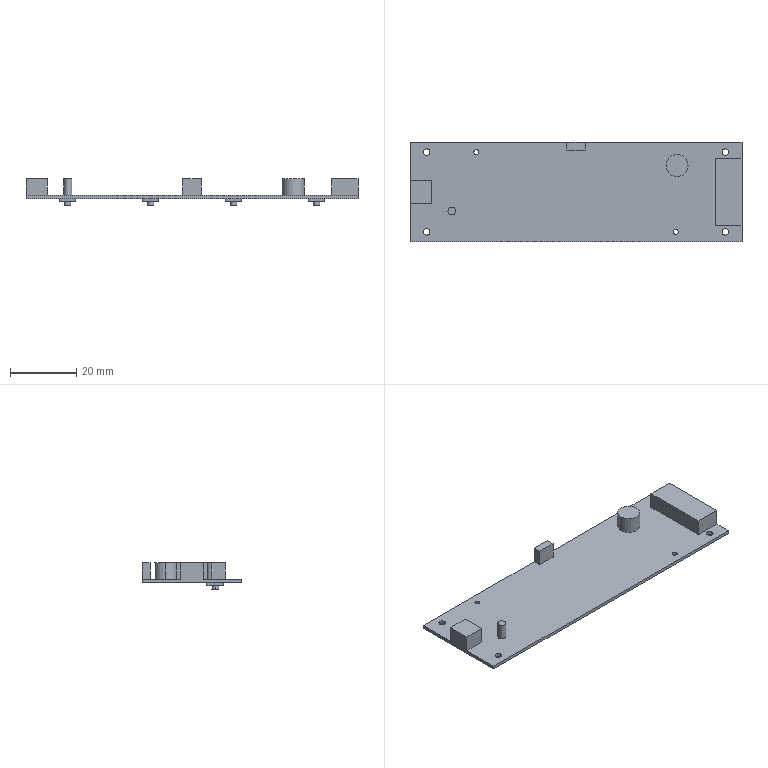Part | SolidWorks | features ICE 4, Extrusion 1 | 1 solid | 68 faces | box 100 x 30 x 8 mm | volume 4377 mm3 | plane 44 | cylinder 24 | commonest cylinder face diameters 2 x16 1.5 x4 2.365 x2 6.624 x2